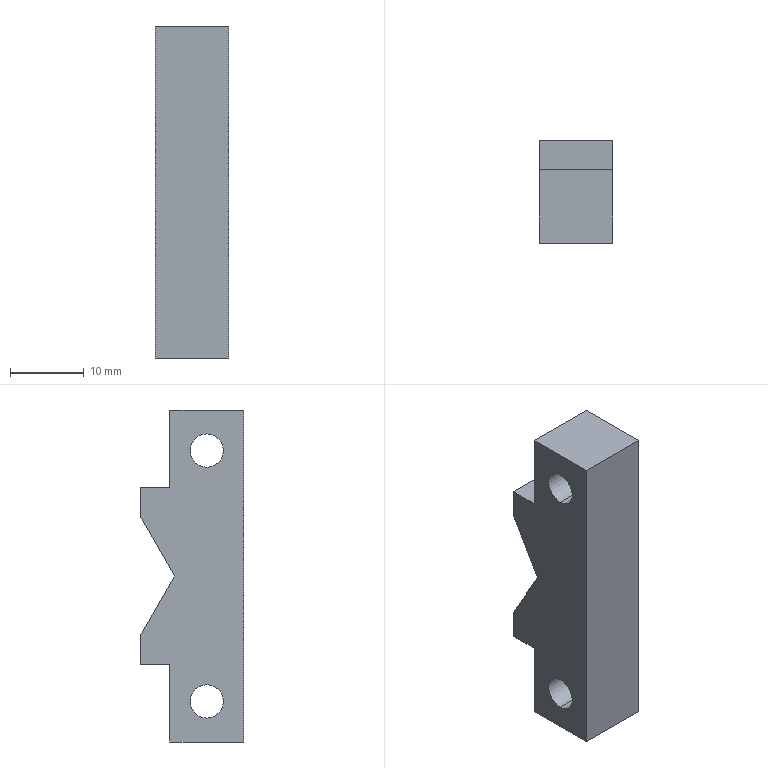Part | STEP file | 02-18 Pull-off block | 1 solid | 23 faces | box 10 x 14 x 45 mm | volume 4364 mm3 | plane 15 | cylinder 8 | commonest cylinder face diameters 4.5 x4 8.5 x4